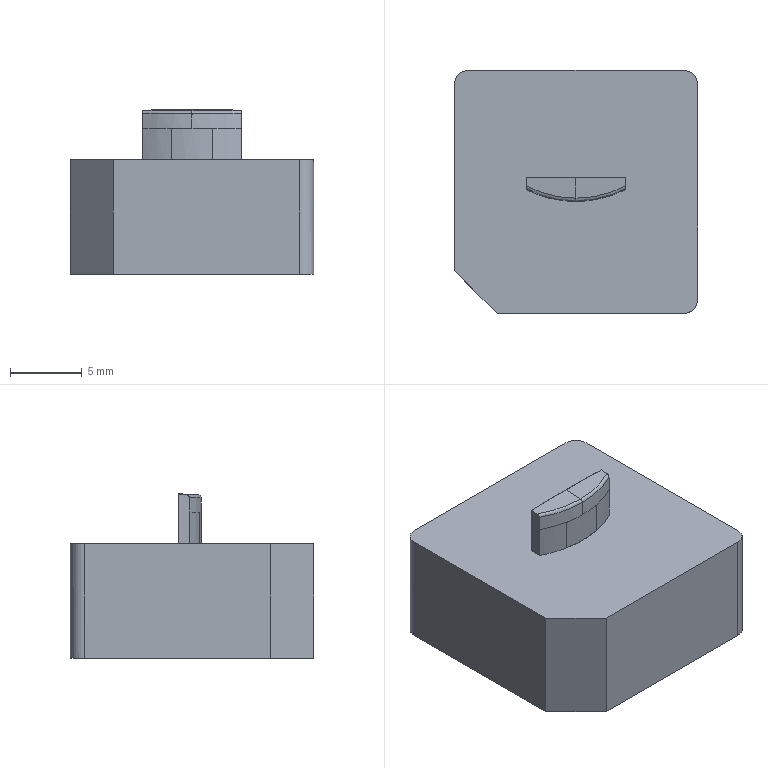NC program | PowerMill | posted with a generic post | part box 17 x 17 x 11.498 mm
Lines 3903 to 4666 of 31087:
N4000 M6
N4001 S18000 M03
N4002 G00 G90 X0.0 Y0.0
N4003 G43 Z10.798 H4
N4004
N4005 G05 P10000 R8
N4006 X3.9989 Y-0.5185
N4007 Z-0.0094
N4008 G01 Z-1.2094 F1200.0
N4009 X3.9866 Y-0.5307 Z-1.2178 F2000.0
N4010 X3.9729 Y-0.5445 Z-1.2349
N4011 X3.9538 Y-0.5635 Z-1.2617
N4012 X3.939 Y-0.5784 Z-1.287
N4013 X3.9276 Y-0.5897 Z-1.3116
N4014 X3.9193 Y-0.598 Z-1.336
N4015 X3.9138 Y-0.6036 Z-1.3609
N4016 X3.8159 Y-0.659 Z-1.426
N4017 X3.82 Y-0.6549 Z-1.3889
N4018 X3.827 Y-0.648 Z-1.3504
N4019 X3.8368 Y-0.6381 Z-1.3118
N4020 X3.8491 Y-0.6258 Z-1.2744
N4021 X3.8638 Y-0.6111 Z-1.2391
N4022 X3.8804 Y-0.5945 Z-1.2067
N4023 X3.8987 Y-0.5762 Z-1.1775
N4024 X3.9184 Y-0.5565 Z-1.1517
N4025 X3.9394 Y-0.5356 Z-1.1294
N4026 X3.9615 Y-0.5134 Z-1.1107
N4027 X3.9664 Y-0.5085 Z-1.1071
N4028 X3.9983 Y-0.4766 Z-1.0915
N4029 X3.9929 Y-0.4396 Z-1.0071
N4030 X3.9712 Y-0.4613 Z-1.013
N4031 X3.9454 Y-0.4871 Z-1.0266
N4032 X3.9195 Y-0.513 Z-1.0442
N4033 X3.8946 Y-0.5379 Z-1.0654
N4034 X3.8706 Y-0.5619 Z-1.0903
N4035 X3.8476 Y-0.5849 Z-1.1192
N4036 X3.8255 Y-0.607 Z-1.1521
N4037 X3.8043 Y-0.6282 Z-1.1894
N4038 X3.7839 Y-0.6486 Z-1.2313
N4039 X3.7729 Y-0.6596 Z-1.2568
N4040 X3.7625 Y-0.67 Z-1.2827
N4041 X3.7532 Y-0.6793 Z-1.3095
N4042 X3.7457 Y-0.6868 Z-1.3373
N4043 X3.7402 Y-0.6923 Z-1.3665
N4044 X3.7364 Y-0.6961 Z-1.3961
N4045 X3.7334 Y-0.6991 Z-1.4258
N4046 X3.7308 Y-0.7017 Z-1.4554
N4047 X3.6483 Y-0.7418 Z-1.4755
N4048 X3.6508 Y-0.7393 Z-1.4322
N4049 X3.6557 Y-0.7344 Z-1.39
N4050 X3.6631 Y-0.7269 Z-1.3488
N4051 X3.6732 Y-0.7169 Z-1.3086
N4052 X3.6859 Y-0.7042 Z-1.2694
N4053 X3.7013 Y-0.6887 Z-1.2311
N4054 X3.7197 Y-0.6704 Z-1.1936
N4055 X3.741 Y-0.649 Z-1.1568
N4056 X3.7649 Y-0.6252 Z-1.1206
N4057 X3.794 Y-0.596 Z-1.0798
N4058 X3.8214 Y-0.5687 Z-1.0457
N4059 X3.8478 Y-0.5422 Z-1.0175
N4060 X3.8739 Y-0.5161 Z-0.994
N4061 X3.9002 Y-0.4899 Z-0.9747
N4062 X3.9269 Y-0.4632 Z-0.9591
N4063 X3.9543 Y-0.4357 Z-0.9466
N4064 X3.9603 Y-0.4297 Z-0.9444
N4065 X3.9838 Y-0.4063 Z-0.9397
N4066 X3.9712 Y-0.3765 Z-0.881
N4067 X3.9561 Y-0.3915 Z-0.8839
N4068 X3.9296 Y-0.4181 Z-0.8919
N4069 X3.9022 Y-0.4454 Z-0.9041
N4070 X3.8737 Y-0.474 Z-0.9209
N4071 X3.8434 Y-0.5043 Z-0.9428
N4072 X3.8102 Y-0.5375 Z-0.971
N4073 X3.7907 Y-0.5569 Z-0.9892
N4074 X3.7703 Y-0.5774 Z-1.0101
N4075 X3.7462 Y-0.6014 Z-1.0372
N4076 X3.7175 Y-0.6302 Z-1.0727
N4077 X3.6866 Y-0.661 Z-1.115
N4078 X3.663 Y-0.6846 Z-1.151
N4079 X3.6449 Y-0.7028 Z-1.1819
N4080 X3.6308 Y-0.7168 Z-1.2089
N4081 X3.6195 Y-0.7282 Z-1.2346
N4082 X3.6095 Y-0.7381 Z-1.2617
N4083 X3.5991 Y-0.7485 Z-1.2918
N4084 X3.5896 Y-0.758 Z-1.3224
N4085 X3.582 Y-0.7657 Z-1.354
N4086 X3.5767 Y-0.7709 Z-1.3867
N4087 X3.5734 Y-0.7743 Z-1.42
N4088 X3.5708 Y-0.7768 Z-1.4534
N4089 X3.5685 Y-0.7791 Z-1.4868
N4090 X3.4906 Y-0.8146 Z-1.4933
N4091 X3.4931 Y-0.8121 Z-1.4476
N4092 X3.4977 Y-0.8076 Z-1.4036
N4093 X3.5043 Y-0.8009 Z-1.361
N4094 X3.5133 Y-0.7919 Z-1.3197
N4095 X3.5247 Y-0.7805 Z-1.2797
N4096 X3.5387 Y-0.7665 Z-1.2406
N4097 X3.5555 Y-0.7497 Z-1.2022
N4098 X3.5754 Y-0.7298 Z-1.1643
N4099 X3.5987 Y-0.7065 Z-1.1264
N4100 X3.6255 Y-0.6797 Z-1.0883
N4101 X3.6561 Y-0.6491 Z-1.0495
N4102 X3.6901 Y-0.6151 Z-1.0101
N4103 X3.7296 Y-0.5756 Z-0.9685
N4104 X3.7673 Y-0.5379 Z-0.9332
N4105 X3.8032 Y-0.502 Z-0.9038
N4106 X3.8372 Y-0.468 Z-0.8799
N4107 X3.8697 Y-0.4355 Z-0.8609
N4108 X3.9007 Y-0.4045 Z-0.8466
N4109 X3.9303 Y-0.3749 Z-0.8366
N4110 X3.9582 Y-0.347 Z-0.8309
N4111 X3.9475 Y-0.3153 Z-0.7871
N4112 X3.9319 Y-0.3309 Z-0.7888
N4113 X3.9038 Y-0.3589 Z-0.7944
N4114 X3.8754 Y-0.3874 Z-0.8035
N4115 X3.8461 Y-0.4167 Z-0.8167
N4116 X3.8148 Y-0.448 Z-0.8346
N4117 X3.7801 Y-0.4827 Z-0.8585
N4118 X3.7393 Y-0.5235 Z-0.8902
N4119 X3.6959 Y-0.5668 Z-0.9256
N4120 X3.6544 Y-0.6084 Z-0.9632
N4121 X3.6165 Y-0.6463 Z-1.0018
N4122 X3.5821 Y-0.6807 Z-1.0415
N4123 X3.5508 Y-0.712 Z-1.0825
N4124 X3.5225 Y-0.7403 Z-1.1246
N4125 X3.4995 Y-0.7632 Z-1.1634
N4126 X3.4793 Y-0.7834 Z-1.2027
N4127 X3.462 Y-0.8008 Z-1.2424
N4128 X3.4476 Y-0.8152 Z-1.2827
N4129 X3.436 Y-0.8268 Z-1.3238
N4130 X3.427 Y-0.8358 Z-1.3658
N4131 X3.4206 Y-0.8422 Z-1.409
N4132 X3.4166 Y-0.8462 Z-1.4536
N4133 X3.4147 Y-0.848 Z-1.4996
N4134 X3.3401 Y-0.8802 Z-1.5011
N4135 X3.3421 Y-0.8783 Z-1.456
N4136 X3.346 Y-0.8743 Z-1.4123
N4137 X3.3521 Y-0.8683 Z-1.3698
N4138 X3.3605 Y-0.8599 Z-1.3283
N4139 X3.3715 Y-0.8488 Z-1.2874
N4140 X3.3854 Y-0.835 Z-1.2469
N4141 X3.4023 Y-0.8181 Z-1.2066
N4142 X3.4224 Y-0.798 Z-1.166
N4143 X3.4425 Y-0.7779 Z-1.1302
N4144 X3.4652 Y-0.7551 Z-1.0947
N4145 X3.4908 Y-0.7296 Z-1.0594
N4146 X3.5227 Y-0.6976 Z-1.0199
N4147 X3.558 Y-0.6624 Z-0.9809
N4148 X3.5883 Y-0.6321 Z-0.9505
N4149 X3.6182 Y-0.6021 Z-0.9228
N4150 X3.6662 Y-0.5541 Z-0.8817
N4151 X3.7115 Y-0.5088 Z-0.8469
N4152 X3.7543 Y-0.4661 Z-0.8181
N4153 X3.7753 Y-0.4451 Z-0.8055
N4154 X3.7963 Y-0.424 Z-0.7931
N4155 X3.8175 Y-0.4029 Z-0.7811
N4156 X3.8389 Y-0.3814 Z-0.7699
N4157 X3.8607 Y-0.3596 Z-0.7606
N4158 X3.8831 Y-0.3373 Z-0.7542
N4159 X3.9057 Y-0.3146 Z-0.7502
N4160 X3.9285 Y-0.2919 Z-0.7474
N4161 X3.9365 Y-0.2839 Z-0.7464
N4162 X3.925 Y-0.253 Z-0.708
N4163 X3.8996 Y-0.2783 Z-0.711
N4164 X3.8661 Y-0.3118 Z-0.7184
N4165 X3.831 Y-0.3469 Z-0.7301
N4166 X3.7935 Y-0.3845 Z-0.7465
N4167 X3.7524 Y-0.4255 Z-0.7684
N4168 X3.7053 Y-0.4727 Z-0.7972
N4169 X3.6483 Y-0.5296 Z-0.8358
N4170 X3.5948 Y-0.5831 Z-0.8762
N4171 X3.5531 Y-0.6248 Z-0.911
N4172 X3.5121 Y-0.6659 Z-0.9489
N4173 X3.4731 Y-0.7048 Z-0.9892
N4174 X3.4375 Y-0.7404 Z-1.0306
N4175 X3.4059 Y-0.7721 Z-1.0722
N4176 X3.378 Y-0.7999 Z-1.1136
N4177 X3.3539 Y-0.824 Z-1.1547
N4178 X3.3334 Y-0.8446 Z-1.1954
N4179 X3.3182 Y-0.8597 Z-1.2304
N4180 X3.3041 Y-0.8738 Z-1.2689
N4181 X3.2916 Y-0.8863 Z-1.3107
N4182 X3.2828 Y-0.8952 Z-1.3484
N4183 X3.2771 Y-0.9009 Z-1.383
N4184 X3.2731 Y-0.9048 Z-1.423
N4185 X3.2707 Y-0.9073 Z-1.4584
N4186 X3.2678 Y-0.9101 Z-1.5027
N4187 X3.1957 Y-0.9398 Z-1.5018
N4188 X3.1983 Y-0.9372 Z-1.4562
N4189 X3.2023 Y-0.9332 Z-1.4122
N4190 X3.208 Y-0.9275 Z-1.3696
N4191 X3.2158 Y-0.9197 Z-1.3282
N4192 X3.2259 Y-0.9096 Z-1.2877
N4193 X3.2387 Y-0.8968 Z-1.248
N4194 X3.2543 Y-0.8812 Z-1.2089
N4195 X3.2725 Y-0.863 Z-1.1711
N4196 X3.2928 Y-0.8427 Z-1.1344
N4197 X3.3151 Y-0.8204 Z-1.0985
N4198 X3.3393 Y-0.7962 Z-1.0626
N4199 X3.3718 Y-0.7637 Z-1.0194
N4200 X3.4072 Y-0.7283 Z-0.9779
N4201 X3.4454 Y-0.6902 Z-0.9382
N4202 X3.4863 Y-0.6493 Z-0.9005
N4203 X3.5298 Y-0.6057 Z-0.865
N4204 X3.5756 Y-0.5599 Z-0.8313
N4205 X3.6364 Y-0.4991 Z-0.7895
N4206 X3.6915 Y-0.444 Z-0.7553
N4207 X3.7224 Y-0.4131 Z-0.7378
N4208 X3.7497 Y-0.3858 Z-0.7233
N4209 X3.7771 Y-0.3584 Z-0.7093
N4210 X3.8049 Y-0.3306 Z-0.6967
N4211 X3.8332 Y-0.3023 Z-0.687
N4212 X3.8621 Y-0.2735 Z-0.6809
N4213 X3.8911 Y-0.2444 Z-0.6768
N4214 X3.9132 Y-0.2223 Z-0.6741
N4215 X3.901 Y-0.1921 Z-0.6437
N4216 X3.8845 Y-0.2086 Z-0.6442
N4217 X3.8557 Y-0.2374 Z-0.6471
N4218 X3.8263 Y-0.2668 Z-0.6528
N4219 X3.7952 Y-0.2979 Z-0.6619
N4220 X3.7606 Y-0.3325 Z-0.6757
N4221 X3.72 Y-0.3731 Z-0.6955
N4222 X3.6841 Y-0.409 Z-0.7148
N4223 X3.6508 Y-0.4423 Z-0.7329
N4224 X3.5998 Y-0.4933 Z-0.7621
N4225 X3.5449 Y-0.5482 Z-0.7972
N4226 X3.4904 Y-0.6027 Z-0.8361
N4227 X3.4409 Y-0.6522 Z-0.8754
N4228 X3.3968 Y-0.6963 Z-0.9143
N4229 X3.356 Y-0.7371 Z-0.9544
N4230 X3.3196 Y-0.7735 Z-0.9942
N4231 X3.286 Y-0.8071 Z-1.0353
N4232 X3.2564 Y-0.8367 Z-1.0762
N4233 X3.2304 Y-0.8626 Z-1.1172
N4234 X3.2078 Y-0.8853 Z-1.1585
N4235 X3.1882 Y-0.9049 Z-1.2003
N4236 X3.1759 Y-0.9172 Z-1.2304
N4237 X3.1645 Y-0.9286 Z-1.2612
N4238 X3.1541 Y-0.939 Z-1.2926
N4239 X3.1453 Y-0.9478 Z-1.325
N4240 X3.1383 Y-0.9548 Z-1.3597
N4241 X3.1334 Y-0.9597 Z-1.3956
N4242 X3.1302 Y-0.9629 Z-1.4303
N4243 X3.128 Y-0.9651 Z-1.4651
N4244 X3.1262 Y-0.9669 Z-1.4999
N4245 X3.057 Y-0.9937 Z-1.498
N4246 X3.0593 Y-0.9914 Z-1.4485
N4247 X3.0638 Y-0.9869 Z-1.4008
N4248 X3.0707 Y-0.98 Z-1.3548
N4249 X3.0801 Y-0.9706 Z-1.3103
N4250 X3.0921 Y-0.9585 Z-1.2675
N4251 X3.1067 Y-0.944 Z-1.2261
N4252 X3.1238 Y-0.9269 Z-1.186
N4253 X3.1434 Y-0.9073 Z-1.1468
N4254 X3.169 Y-0.8816 Z-1.1021
N4255 X3.1975 Y-0.8532 Z-1.0587
N4256 X3.229 Y-0.8216 Z-1.0163
N4257 X3.2639 Y-0.7867 Z-0.9748
N4258 X3.3024 Y-0.7482 Z-0.9342
N4259 X3.345 Y-0.7057 Z-0.8941
N4260 X3.391 Y-0.6596 Z-0.8551
N4261 X3.4449 Y-0.6058 Z-0.8139
N4262 X3.4999 Y-0.5507 Z-0.7758
N4263 X3.5584 Y-0.4922 Z-0.7395
N4264 X3.6225 Y-0.4282 Z-0.7037
N4265 X3.6828 Y-0.3679 Z-0.6731
N4266 X3.728 Y-0.3227 Z-0.652
N4267 X3.7693 Y-0.2813 Z-0.636
N4268 X3.8079 Y-0.2427 Z-0.6247
N4269 X3.8444 Y-0.2062 Z-0.6177
N4270 X3.8792 Y-0.1714 Z-0.6147
N4271 X3.8884 Y-0.1623 Z-0.6146
N4272 X3.8779 Y-0.1303 Z-0.5873
N4273 X3.839 Y-0.1692 Z-0.5897
N4274 X3.8009 Y-0.2073 Z-0.5948
N4275 X3.7683 Y-0.24 Z-0.6023
N4276 X3.7397 Y-0.2685 Z-0.6123
N4277 X3.688 Y-0.3202 Z-0.6341
N4278 X3.6299 Y-0.3783 Z-0.6599
N4279 X3.5724 Y-0.4359 Z-0.6881
N4280 X3.5155 Y-0.4927 Z-0.7191
N4281 X3.4713 Y-0.537 Z-0.7455
N4282 X3.4106 Y-0.5976 Z-0.7846
N4283 X3.3562 Y-0.652 Z-0.8236
N4284 X3.3069 Y-0.7013 Z-0.8628
N4285 X3.2621 Y-0.7462 Z-0.9027
N4286 X3.2212 Y-0.787 Z-0.9434
N4287 X3.1835 Y-0.8248 Z-0.9855
N4288 X3.149 Y-0.8592 Z-1.0284
N4289 X3.1191 Y-0.8891 Z-1.0703
N4290 X3.0931 Y-0.9151 Z-1.1119
N4291 X3.0705 Y-0.9377 Z-1.1534
N4292 X3.0539 Y-0.9543 Z-1.1887
N4293 X3.039 Y-0.9692 Z-1.2239
N4294 X3.0255 Y-0.9828 Z-1.261
N4295 X3.0137 Y-0.9945 Z-1.3007
N4296 X3.0048 Y-1.0034 Z-1.3404
N4297 X2.9984 Y-1.0098 Z-1.3795
N4298 X2.994 Y-1.0142 Z-1.4184
N4299 X2.991 Y-1.0173 Z-1.4578
N4300 X2.989 Y-1.0193 Z-1.4983
N4301 X2.9222 Y-1.0436 Z-1.4995
N4302 X2.9241 Y-1.0417 Z-1.4521
N4303 X2.9281 Y-1.0377 Z-1.4061
N4304 X2.9342 Y-1.0316 Z-1.3615
N4305 X2.9427 Y-1.0231 Z-1.3179
N4306 X2.9537 Y-1.0121 Z-1.2754
N4307 X2.9674 Y-0.9984 Z-1.2335
N4308 X2.984 Y-0.9818 Z-1.192
N4309 X3.0038 Y-0.962 Z-1.1506
N4310 X3.0268 Y-0.939 Z-1.109
N4311 X3.0533 Y-0.9125 Z-1.0669
N4312 X3.0828 Y-0.883 Z-1.0248
N4313 X3.1166 Y-0.8492 Z-0.982
N4314 X3.1538 Y-0.812 Z-0.9401
N4315 X3.1947 Y-0.7711 Z-0.8991
N4316 X3.2396 Y-0.7262 Z-0.8588
N4317 X3.2889 Y-0.6769 Z-0.819
N4318 X3.3433 Y-0.6225 Z-0.7797
N4319 X3.3936 Y-0.5722 Z-0.7465
N4320 X3.4586 Y-0.5072 Z-0.7075
N4321 X3.5242 Y-0.4416 Z-0.6725
N4322 X3.584 Y-0.3818 Z-0.6443
N4323 X3.6049 Y-0.3609 Z-0.635
N4324 X3.6259 Y-0.3399 Z-0.6257
N4325 X3.6524 Y-0.3134 Z-0.6141
N4326 X3.6735 Y-0.2923 Z-0.6052
N4327 X3.6946 Y-0.2712 Z-0.5966
N4328 X3.7158 Y-0.25 Z-0.5889
N4329 X3.7418 Y-0.224 Z-0.5808
N4330 X3.768 Y-0.1978 Z-0.5734
N4331 X3.7963 Y-0.1695 Z-0.567
N4332 X3.8264 Y-0.1394 Z-0.5631
N4333 X3.853 Y-0.1128 Z-0.5627
N4334 X3.8667 Y-0.0991 Z-0.5635
N4335 X3.8552 Y-0.0682 Z-0.5403
N4336 X3.8333 Y-0.0901 Z-0.5405
N4337 X3.8048 Y-0.1186 Z-0.5413
N4338 X3.7763 Y-0.147 Z-0.5441
N4339 X3.7482 Y-0.1752 Z-0.5501
N4340 X3.7203 Y-0.2031 Z-0.5584
N4341 X3.6925 Y-0.2309 Z-0.5677
N4342 X3.6648 Y-0.2585 Z-0.5773
N4343 X3.6068 Y-0.3166 Z-0.5995
N4344 X3.5382 Y-0.3852 Z-0.6294
N4345 X3.4809 Y-0.4424 Z-0.6561
N4346 X3.426 Y-0.4974 Z-0.6831
N4347 X3.3686 Y-0.5547 Z-0.7149
N4348 X3.3098 Y-0.6136 Z-0.7516
N4349 X3.2532 Y-0.6702 Z-0.791
N4350 X3.2006 Y-0.7228 Z-0.8319
N4351 X3.1524 Y-0.7709 Z-0.8733
N4352 X3.1075 Y-0.8159 Z-0.9162
N4353 X3.0762 Y-0.8472 Z-0.949
N4354 X3.0396 Y-0.8838 Z-0.991
N4355 X3.0074 Y-0.9159 Z-1.0327
N4356 X2.9791 Y-0.9443 Z-1.0743
N4357 X2.9541 Y-0.9693 Z-1.1162
N4358 X2.9323 Y-0.9911 Z-1.1587
N4359 X2.9134 Y-1.01 Z-1.2018
N4360 X2.8971 Y-1.0262 Z-1.2462
N4361 X2.8878 Y-1.0356 Z-1.2758
N4362 X2.8793 Y-1.0441 Z-1.3057
N4363 X2.872 Y-1.0514 Z-1.3363
N4364 X2.8664 Y-1.057 Z-1.3676
N4365 X2.8621 Y-1.0613 Z-1.4035
N4366 X2.8595 Y-1.0639 Z-1.4359
N4367 X2.8575 Y-1.0659 Z-1.4683
N4368 X2.8555 Y-1.0678 Z-1.5007
N4369 X2.7907 Y-1.0903 Z-1.5072
N4370 X2.7921 Y-1.0888 Z-1.4595
N4371 X2.7957 Y-1.0852 Z-1.413
N4372 X2.8016 Y-1.0793 Z-1.3676
N4373 X2.81 Y-1.071 Z-1.3232
N4374 X2.8209 Y-1.0601 Z-1.2795
N4375 X2.8345 Y-1.0464 Z-1.2365
N4376 X2.851 Y-1.0299 Z-1.1937
N4377 X2.8707 Y-1.0102 Z-1.1509
N4378 X2.8939 Y-0.987 Z-1.1076
N4379 X2.9209 Y-0.96 Z-1.0634
N4380 X2.9514 Y-0.9295 Z-1.019
N4381 X2.985 Y-0.896 Z-0.9758
N4382 X3.0219 Y-0.8591 Z-0.9335
N4383 X3.0624 Y-0.8186 Z-0.8922
N4384 X3.1069 Y-0.7741 Z-0.8515
N4385 X3.1557 Y-0.7252 Z-0.8115
N4386 X3.2093 Y-0.6717 Z-0.772
N4387 X3.2551 Y-0.6259 Z-0.7413
N4388 X3.3205 Y-0.5605 Z-0.7011
N4389 X3.3843 Y-0.4967 Z-0.666
N4390 X3.4452 Y-0.4358 Z-0.6364
N4391 X3.4752 Y-0.4057 Z-0.623
N4392 X3.5054 Y-0.3756 Z-0.6099
N4393 X3.5355 Y-0.3454 Z-0.5972
N4394 X3.5721 Y-0.3088 Z-0.5821
N4395 X3.6176 Y-0.2634 Z-0.5642
N4396 X3.648 Y-0.233 Z-0.5529
N4397 X3.6786 Y-0.2024 Z-0.5425
N4398 X3.7091 Y-0.1718 Z-0.5337
N4399 X3.7544 Y-0.1266 Z-0.524
N4400 X3.792 Y-0.089 Z-0.5188
N4401 X3.8252 Y-0.0558 Z-0.5175
N4402 X3.8442 Y-0.0367 Z-0.5186
N4403 X3.8319 Y-0.0066 Z-0.4999
N4404 X3.8316 Y-0.0069
N4405 X3.7837 Y-0.0548
N4406 X3.7449 Y-0.0936 Z-0.5027
N4407 X3.7202 Y-0.1183 Z-0.5065
N4408 X3.6957 Y-0.1428 Z-0.5124
N4409 X3.6713 Y-0.1672 Z-0.5194
N4410 X3.6375 Y-0.201 Z-0.5299
N4411 X3.6133 Y-0.2253 Z-0.5379
N4412 X3.5891 Y-0.2495 Z-0.5461
N4413 X3.5602 Y-0.2783 Z-0.5563
N4414 X3.4932 Y-0.3453 Z-0.5815
N4415 X3.4268 Y-0.4117 Z-0.6095
N4416 X3.3611 Y-0.4774 Z-0.6406
N4417 X3.3067 Y-0.5318 Z-0.6683
N4418 X3.2419 Y-0.5966 Z-0.7045
N4419 X3.1817 Y-0.6568 Z-0.742
N4420 X3.1256 Y-0.7129 Z-0.781
N4421 X3.073 Y-0.7655 Z-0.8217
N4422 X3.0237 Y-0.8148 Z-0.8643
N4423 X2.9815 Y-0.857 Z-0.9047
N4424 X2.9423 Y-0.8962 Z-0.9466
N4425 X2.907 Y-0.9315 Z-0.9888
N4426 X2.8757 Y-0.9628 Z-1.0311
N4427 X2.8481 Y-0.9904 Z-1.0734
N4428 X2.8276 Y-1.0109 Z-1.109
N4429 X2.8091 Y-1.0294 Z-1.1444
N4430 X2.792 Y-1.0465 Z-1.1803
N4431 X2.7765 Y-1.062 Z-1.2173
N4432 X2.7628 Y-1.0757 Z-1.2562
N4433 X2.7512 Y-1.0873 Z-1.2973
N4434 X2.7421 Y-1.0964 Z-1.3398
N4435 X2.7356 Y-1.103 Z-1.3824
N4436 X2.731 Y-1.1075 Z-1.4255
N4437 X2.7279 Y-1.1106 Z-1.4693
N4438 X2.726 Y-1.1126 Z-1.5141
N4439 X2.6622 Y-1.1339 Z-1.5167
N4440 X2.6642 Y-1.1319 Z-1.468
N4441 X2.6677 Y-1.1284 Z-1.421
N4442 X2.6731 Y-1.123 Z-1.3754
N4443 X2.6805 Y-1.1156 Z-1.331
N4444 X2.6902 Y-1.1059 Z-1.2877
N4445 X2.7025 Y-1.0936 Z-1.2452
N4446 X2.7175 Y-1.0785 Z-1.2032
N4447 X2.7356 Y-1.0605 Z-1.1616
N4448 X2.7567 Y-1.0394 Z-1.1202
N4449 X2.7802 Y-1.0159 Z-1.0796
N4450 X2.8058 Y-0.9903 Z-1.0395
N4451 X2.8335 Y-0.9626 Z-1.0
N4452 X2.8676 Y-0.9285 Z-0.9567
N4453 X2.9046 Y-0.8915 Z-0.915
N4454 X2.9446 Y-0.8515 Z-0.8749
N4455 X2.9875 Y-0.8086 Z-0.8364
N4456 X3.04 Y-0.7561 Z-0.7936
N4457 X3.0953 Y-0.7008 Z-0.7531
N4458 X3.154 Y-0.6421 Z-0.7144
N4459 X3.2167 Y-0.5794 Z-0.6775
N4460 X3.2839 Y-0.5122 Z-0.642
N4461 X3.3567 Y-0.4394 Z-0.6076
N4462 X3.4341 Y-0.362 Z-0.5746
N4463 X3.505 Y-0.2911 Z-0.5479
N4464 X3.5263 Y-0.2698 Z-0.5406
N4465 X3.5476 Y-0.2485 Z-0.5334
N4466 X3.5689 Y-0.2272 Z-0.5263
N4467 X3.5975 Y-0.1986 Z-0.5169
N4468 X3.6189 Y-0.1772 Z-0.51
N4469 X3.6403 Y-0.1558 Z-0.5035
N4470 X3.6619 Y-0.1342 Z-0.4979
N4471 X3.6836 Y-0.1125 Z-0.4929
N4472 X3.7055 Y-0.0906 Z-0.488
N4473 X3.7273 Y-0.0688 Z-0.4835
N4474 X3.7493 Y-0.0468 Z-0.48
N4475 X3.7713 Y-0.0248 Z-0.4787
N4476 X3.7934 Y-0.0027 Z-0.4796
N4477 X3.8154 Y0.0193 Z-0.4814
N4478 X3.8198 Y0.0237 Z-0.4818
N4479 X3.8081 Y0.0544 Z-0.4642
N4480 X3.8053 Y0.0516 Z-0.4637
N4481 X3.7769 Y0.0232 Z-0.4612
N4482 X3.7452 Y-0.0084 Z-0.4622
N4483 X3.7089 Y-0.0448 Z-0.467
N4484 X3.6634 Y-0.0903 Z-0.4765
N4485 X3.5837 Y-0.17 Z-0.4968
N4486 X3.5035 Y-0.2501 Z-0.5213
N4487 X3.4206 Y-0.3331 Z-0.5506
N4488 X3.3394 Y-0.4142 Z-0.5828
N4489 X3.287 Y-0.4666 Z-0.6055
N4490 X3.222 Y-0.5316 Z-0.6364
N4491 X3.1564 Y-0.5973 Z-0.671
N4492 X3.0937 Y-0.6599 Z-0.7079
N4493 X3.0353 Y-0.7184 Z-0.7462
N4494 X2.9813 Y-0.7724 Z-0.7856
N4495 X2.9315 Y-0.8221 Z-0.826
N4496 X2.8859 Y-0.8678 Z-0.8674
N4497 X2.8441 Y-0.9096 Z-0.9096
N4498 X2.8059 Y-0.9478 Z-0.9527
N4499 X2.7711 Y-0.9826 Z-0.9967
N4500 X2.7396 Y-1.0141 Z-1.0416
N4501 X2.7112 Y-1.0424 Z-1.0874
N4502 X2.6903 Y-1.0633 Z-1.1252
N4503 X2.6713 Y-1.0823 Z-1.1635
N4504 X2.6543 Y-1.0993 Z-1.2029
N4505 X2.6395 Y-1.1141 Z-1.2438
N4506 X2.6272 Y-1.1265 Z-1.2864
N4507 X2.6175 Y-1.1362 Z-1.3302
N4508 X2.6102 Y-1.1434 Z-1.3748
N4509 X2.6052 Y-1.1485 Z-1.4204
N4510 X2.6019 Y-1.1517 Z-1.4672
N4511 X2.6001 Y-1.1535 Z-1.5153
N4512 X2.5381 Y-1.1731 Z-1.5135
N4513 X2.54 Y-1.1713 Z-1.4794
N4514 X2.5419 Y-1.1693 Z-1.4446
N4515 X2.5447 Y-1.1666 Z-1.4068
N4516 X2.5494 Y-1.1618 Z-1.3649
N4517 X2.5553 Y-1.156 Z-1.3309
N4518 X2.5624 Y-1.1489 Z-1.2994
N4519 X2.5708 Y-1.1404 Z-1.2685
N4520 X2.5803 Y-1.1309 Z-1.2381
N4521 X2.5973 Y-1.1139 Z-1.1917
N4522 X2.6171 Y-1.0941 Z-1.146
N4523 X2.64 Y-1.0713 Z-1.1009
N4524 X2.6659 Y-1.0453 Z-1.0563
N4525 X2.6951 Y-1.0162 Z-1.0124
N4526 X2.7277 Y-0.9835 Z-0.9689
N4527 X2.764 Y-0.9472 Z-0.926
N4528 X2.8042 Y-0.907 Z-0.8835
N4529 X2.8485 Y-0.8628 Z-0.8414
N4530 X2.8969 Y-0.8143 Z-0.8
N4531 X2.949 Y-0.7623 Z-0.7598
N4532 X3.0036 Y-0.7076 Z-0.7217
N4533 X3.063 Y-0.6482 Z-0.6846
N4534 X3.1269 Y-0.5844 Z-0.6489
N4535 X3.1958 Y-0.5154 Z-0.6146
N4536 X3.2711 Y-0.4402 Z-0.5809
N4537 X3.3548 Y-0.3564 Z-0.5472
N4538 X3.4323 Y-0.279 Z-0.5196
N4539 X3.5167 Y-0.1946 Z-0.4934
N4540 X3.5988 Y-0.1125 Z-0.4702
N4541 X3.6482 Y-0.0631 Z-0.4584
N4542 X3.6951 Y-0.0162 Z-0.4509
N4543 X3.74 Y0.0288 Z-0.4475
N4544 X3.7838 Y0.0725 Z-0.4479
N4545 X3.7959 Y0.0846 Z-0.4487
N4546 X3.784 Y0.1152 Z-0.435
N4547 X3.7525 Y0.0837 Z-0.4335
N4548 X3.7067 Y0.0379 Z-0.4333
N4549 X3.6683 Y-0.0005 Z-0.436
N4550 X3.6453 Y-0.0235 Z-0.4398
N4551 X3.6224 Y-0.0464 Z-0.4448
N4552 X3.5995 Y-0.0693 Z-0.4502
N4553 X3.5704 Y-0.0984 Z-0.4575
N4554 X3.5476 Y-0.1213 Z-0.4633
N4555 X3.5247 Y-0.1441 Z-0.469
N4556 X3.4764 Y-0.1924 Z-0.482
N4557 X3.4283 Y-0.2405 Z-0.4966
N4558 X3.3804 Y-0.2885 Z-0.5121
N4559 X3.3325 Y-0.3363 Z-0.5284
N4560 X3.2848 Y-0.384 Z-0.5456
N4561 X3.2374 Y-0.4314 Z-0.5642
N4562 X3.1607 Y-0.5081 Z-0.5975
N4563 X3.0881 Y-0.5807 Z-0.6329
N4564 X3.0193 Y-0.6495 Z-0.6704
N4565 X2.954 Y-0.7148 Z-0.7102
N4566 X2.9119 Y-0.7569 Z-0.7382
N4567 X2.8665 Y-0.8023 Z-0.7716
N4568 X2.8171 Y-0.8517 Z-0.8116
N4569 X2.7697 Y-0.8991 Z-0.8542
N4570 X2.728 Y-0.9408 Z-0.8957
N4571 X2.6919 Y-0.9769 Z-0.9356
N4572 X2.6589 Y-1.0099 Z-0.9763
N4573 X2.6328 Y-1.036 Z-1.012
N4574 X2.6034 Y-1.0655 Z-1.057
N4575 X2.5774 Y-1.0914 Z-1.102
N4576 X2.5548 Y-1.1141 Z-1.1472
N4577 X2.5353 Y-1.1336 Z-1.1926
N4578 X2.5187 Y-1.1501 Z-1.2383
N4579 X2.5093 Y-1.1595 Z-1.2691
N4580 X2.5009 Y-1.168 Z-1.3005
N4581 X2.4937 Y-1.1751 Z-1.3325
N4582 X2.4882 Y-1.1806 Z-1.3651
N4583 X2.4836 Y-1.1852 Z-1.405
N4584 X2.4808 Y-1.188 Z-1.4436
N4585 X2.4789 Y-1.1899 Z-1.4782
N4586 X2.4772 Y-1.1917 Z-1.5118
N4587 X2.417 Y-1.2094 Z-1.5124
N4588 X2.4189 Y-1.2075 Z-1.4757
N4589 X2.421 Y-1.2054 Z-1.4395
N4590 X2.4237 Y-1.2027 Z-1.4032
N4591 X2.4278 Y-1.1986 Z-1.3652
N4592 X2.4344 Y-1.192 Z-1.3243
N4593 X2.4425 Y-1.1839 Z-1.2887
N4594 X2.4521 Y-1.1743 Z-1.2554
N4595 X2.4632 Y-1.1632 Z-1.223
N4596 X2.4753 Y-1.1511 Z-1.1912
N4597 X2.4883 Y-1.1381 Z-1.1597
N4598 X2.5099 Y-1.1165 Z-1.1138
N4599 X2.5344 Y-1.0919 Z-1.0685
N4600 X2.5621 Y-1.0642 Z-1.024
N4601 X2.5931 Y-1.0333 Z-0.9801
N4602 X2.6275 Y-0.9988 Z-0.9368
N4603 X2.6656 Y-0.9608 Z-0.8942
N4604 X2.7077 Y-0.9187 Z-0.852
N4605 X2.7539 Y-0.8725 Z-0.8104
N4606 X2.8047 Y-0.8217 Z-0.7693
N4607 X2.86 Y-0.7664 Z-0.7289
N4608 X2.9179 Y-0.7085 Z-0.6907
N4609 X2.9796 Y-0.6468 Z-0.6541
N4610 X3.0467 Y-0.5797 Z-0.6183
N4611 X3.1187 Y-0.5077 Z-0.5841
N4612 X3.194 Y-0.4324 Z-0.5524
N4613 X3.2667 Y-0.3597 Z-0.5254
N4614 X3.3312 Y-0.2952 Z-0.5037
N4615 X3.4176 Y-0.2087 Z-0.4772
N4616 X3.5046 Y-0.1218 Z-0.454
N4617 X3.5918 Y-0.0346 Z-0.4336
N4618 X3.635 Y0.0086 Z-0.4248
N4619 X3.677 Y0.0506 Z-0.4192
N4620 X3.7155 Y0.0891 Z-0.4177
N4621 X3.7513 Y0.1249 Z-0.4198
N4622 X3.7721 Y0.1457 Z-0.4228
N4623 X3.76 Y0.176 Z-0.4107
N4624 X3.743 Y0.159 Z-0.4087
N4625 X3.7153 Y0.1313 Z-0.4059
N4626 X3.6876 Y0.1036 Z-0.4049
N4627 X3.6599 Y0.0759 Z-0.4067
N4628 X3.6323 Y0.0483 Z-0.4104
N4629 X3.6047 Y0.0207 Z-0.4149
N4630 X3.5772 Y-0.0068 Z-0.4196
N4631 X3.5171 Y-0.0668 Z-0.4316
N4632 X3.4416 Y-0.1424 Z-0.4501
N4633 X3.3638 Y-0.2202 Z-0.471
N4634 X3.2847 Y-0.2993 Z-0.4943
N4635 X3.2016 Y-0.3824 Z-0.5223
N4636 X3.1205 Y-0.4635 Z-0.5534
N4637 X3.0441 Y-0.5398 Z-0.5865
N4638 X2.9735 Y-0.6105 Z-0.621
N4639 X2.9083 Y-0.6756 Z-0.6564
N4640 X2.8487 Y-0.7353 Z-0.6925
N4641 X2.7918 Y-0.7922 Z-0.7306
N4642 X2.7384 Y-0.8456 Z-0.7703
N4643 X2.689 Y-0.895 Z-0.811
N4644 X2.6437 Y-0.9403 Z-0.8527
N4645 X2.6022 Y-0.9818 Z-0.8952
N4646 X2.5644 Y-1.0195 Z-0.9384
N4647 X2.5301 Y-1.0538 Z-0.9825
N4648 X2.4992 Y-1.0848 Z-1.0274
N4649 X2.4713 Y-1.1127 Z-1.0732
N4650 X2.4465 Y-1.1375 Z-1.1198
N4651 X2.4283 Y-1.1556 Z-1.1585
N4652 X2.4122 Y-1.1718 Z-1.1973
N4653 X2.3978 Y-1.1861 Z-1.2374
N4654 X2.3854 Y-1.1985 Z-1.2795
N4655 X2.3752 Y-1.2088 Z-1.3239
N4656 X2.3674 Y-1.2165 Z-1.3704
N4657 X2.3621 Y-1.2219 Z-1.4175
N4658 X2.3587 Y-1.2253 Z-1.4651
N4659 X2.3569 Y-1.2271 Z-1.5133
N4660 X2.298 Y-1.2436 Z-1.5143
N4661 X2.2996 Y-1.2419 Z-1.4683
N4662 X2.3026 Y-1.2389 Z-1.4229
N4663 X2.3073 Y-1.2342 Z-1.3776
N4664 X2.3143 Y-1.2272 Z-1.3322
N4665 X2.3239 Y-1.2176 Z-1.2878
N4666 X2.3356 Y-1.2059 Z-1.2462
N4667 X2.3492 Y-1.1923 Z-1.2067
N4668 X2.3644 Y-1.1772 Z-1.1687
N4669 X2.3811 Y-1.1605 Z-1.1312
N4670 X2.4037 Y-1.1378 Z-1.0859
N4671 X2.4286 Y-1.1129 Z-1.0424
N4672 X2.4565 Y-1.0851 Z-0.9997
N4673 X2.4879 Y-1.0536 Z-0.9572
N4674 X2.5234 Y-1.0182 Z-0.9146
N4675 X2.5621 Y-0.9795 Z-0.8726
N4676 X2.605 Y-0.9366 Z-0.8303
N4677 X2.6516 Y-0.8899 Z-0.789
N4678 X2.7023 Y-0.8393 Z-0.7488
N4679 X2.7572 Y-0.7843 Z-0.7095
N4680 X2.8167 Y-0.7248 Z-0.6714
N4681 X2.8807 Y-0.6609 Z-0.6347
N4682 X2.9486 Y-0.5929 Z-0.5998
N4683 X3.0189 Y-0.5226 Z-0.5675
N4684 X3.0983 Y-0.4433 Z-0.5349
N4685 X3.1821 Y-0.3595 Z-0.5047
N4686 X3.271 Y-0.2706 Z-0.4766
N4687 X3.3659 Y-0.1756 Z-0.4506
N4688 X3.4681 Y-0.0734 Z-0.426
N4689 X3.5482 Y0.0067 Z-0.4095
N4690 X3.5873 Y0.0458 Z-0.4027
N4691 X3.6156 Y0.0741 Z-0.3984
N4692 X3.644 Y0.1024 Z-0.395
N4693 X3.6724 Y0.1308 Z-0.3933
N4694 X3.7008 Y0.1593 Z-0.3941
N4695 X3.7292 Y0.1876 Z-0.3973
N4696 X3.7477 Y0.2062 Z-0.4003
N4697 X3.7367 Y0.2376 Z-0.3909
N4698 X3.7201 Y0.221 Z-0.388
N4699 X3.6842 Y0.1851 Z-0.3843
N4700 X3.6443 Y0.1452 Z-0.3841
N4701 X3.5981 Y0.099 Z-0.3875
N4702 X3.5772 Y0.0781 Z-0.39
N4703 X3.5564 Y0.0573 Z-0.3935
N4704 X3.5356 Y0.0364 Z-0.3973
N4705 X3.5147 Y0.0156 Z-0.4012
N4706 X3.4902 Y-0.0089 Z-0.406
N4707 X3.4694 Y-0.0297 Z-0.41
N4708 X3.4486 Y-0.0505 Z-0.4142
N4709 X3.4104 Y-0.0887 Z-0.4222
N4710 X3.3098 Y-0.1893 Z-0.4455
N4711 X3.2162 Y-0.283 Z-0.471
N4712 X3.1282 Y-0.3709 Z-0.4986
N4713 X3.045 Y-0.4541 Z-0.5285
N4714 X2.9662 Y-0.5329 Z-0.5607
N4715 X2.8911 Y-0.608 Z-0.5953
N4716 X2.8266 Y-0.6726 Z-0.6285
N4717 X2.7637 Y-0.7354 Z-0.6643
N4718 X2.7043 Y-0.7948 Z-0.702
N4719 X2.6489 Y-0.8502 Z-0.7411
N4720 X2.5978 Y-0.9014 Z-0.7813
N4721 X2.5506 Y-0.9485 Z-0.8226
N4722 X2.5073 Y-0.9918 Z-0.8649
N4723 X2.4676 Y-1.0316 Z-0.9082
N4724 X2.4312 Y-1.0679 Z-0.9525
N4725 X2.3982 Y-1.1009 Z-0.9978
N4726 X2.3682 Y-1.1309 Z-1.0441
N4727 X2.3421 Y-1.1571 Z-1.0899
N4728 X2.3193 Y-1.1799 Z-1.1353
N4729 X2.2997 Y-1.1994 Z-1.1805
N4730 X2.2832 Y-1.2159 Z-1.2258
N4731 X2.2696 Y-1.2295 Z-1.2716
N4732 X2.2588 Y-1.2403 Z-1.318
N4733 X2.2505 Y-1.2486 Z-1.3652
N4734 X2.2446 Y-1.2545 Z-1.4134
N4735 X2.2411 Y-1.258 Z-1.4629
N4736 X2.2397 Y-1.2594 Z-1.5136
N4737 X2.1816 Y-1.2751 Z-1.512
N4738 X2.1833 Y-1.2734 Z-1.4598
N4739 X2.1873 Y-1.2694 Z-1.4089
N4740 X2.1937 Y-1.263 Z-1.3593
N4741 X2.2025 Y-1.2542 Z-1.3109
N4742 X2.2139 Y-1.2428 Z-1.2634
N4743 X2.228 Y-1.2287 Z-1.2169
N4744 X2.2449 Y-1.2117 Z-1.171
N4745 X2.2648 Y-1.1919 Z-1.1258
N4746 X2.2877 Y-1.1689 Z-1.0808
N4747 X2.3139 Y-1.1428 Z-1.036
N4748 X2.3435 Y-1.1132 Z-0.9911
N4749 X2.3762 Y-1.0804 Z-0.9466
N4750 X2.4131 Y-1.0436 Z-0.9019
N4751 X2.4533 Y-1.0034 Z-0.8583
N4752 X2.497 Y-0.9597 Z-0.8157
N4753 X2.5444 Y-0.9123 Z-0.7743
N4754 X2.5958 Y-0.8609 Z-0.734
N4755 X2.6513 Y-0.8054 Z-0.6949
N4756 X2.7111 Y-0.7456 Z-0.6571
N4757 X2.775 Y-0.6817 Z-0.6209
N4758 X2.842 Y-0.6147 Z-0.5869
N4759 X2.9102 Y-0.5465 Z-0.5558
N4760 X2.9878 Y-0.4689 Z-0.5243
N4761 X3.0706 Y-0.386 Z-0.4948
N4762 X3.1597 Y-0.297 Z-0.467
N4763 X3.2563 Y-0.2003 Z-0.4408